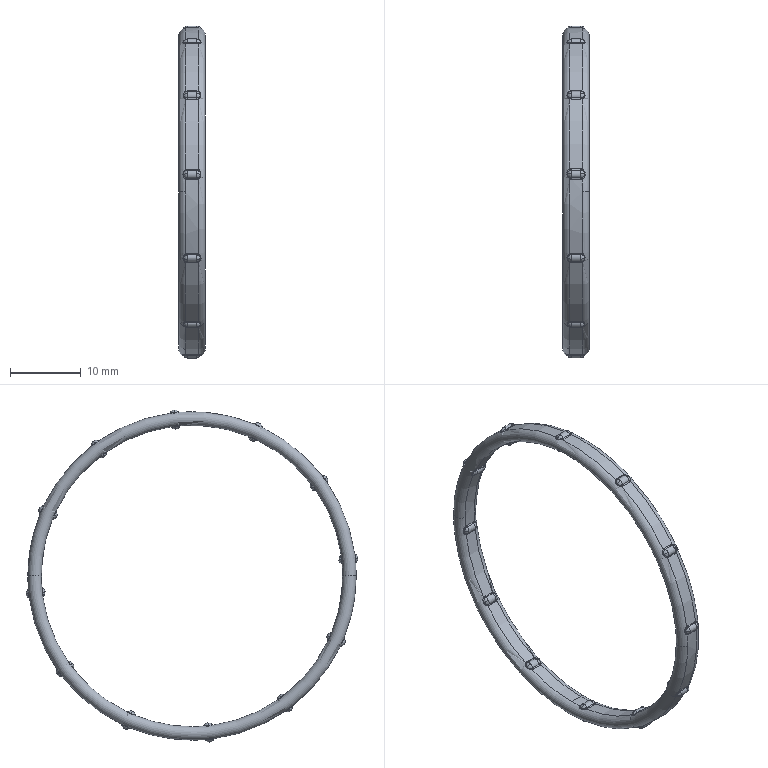Part | NX | features BREP 1 | 1 solid | 358 faces | box 3.7 x 46.932 x 46.932 mm | volume 892.47 mm3 | spline 240 | cylinder 114 | torus 4 | commonest cylinder face diameters 0.4 x56 1.3 x32 42.6 x13 46.4 x13